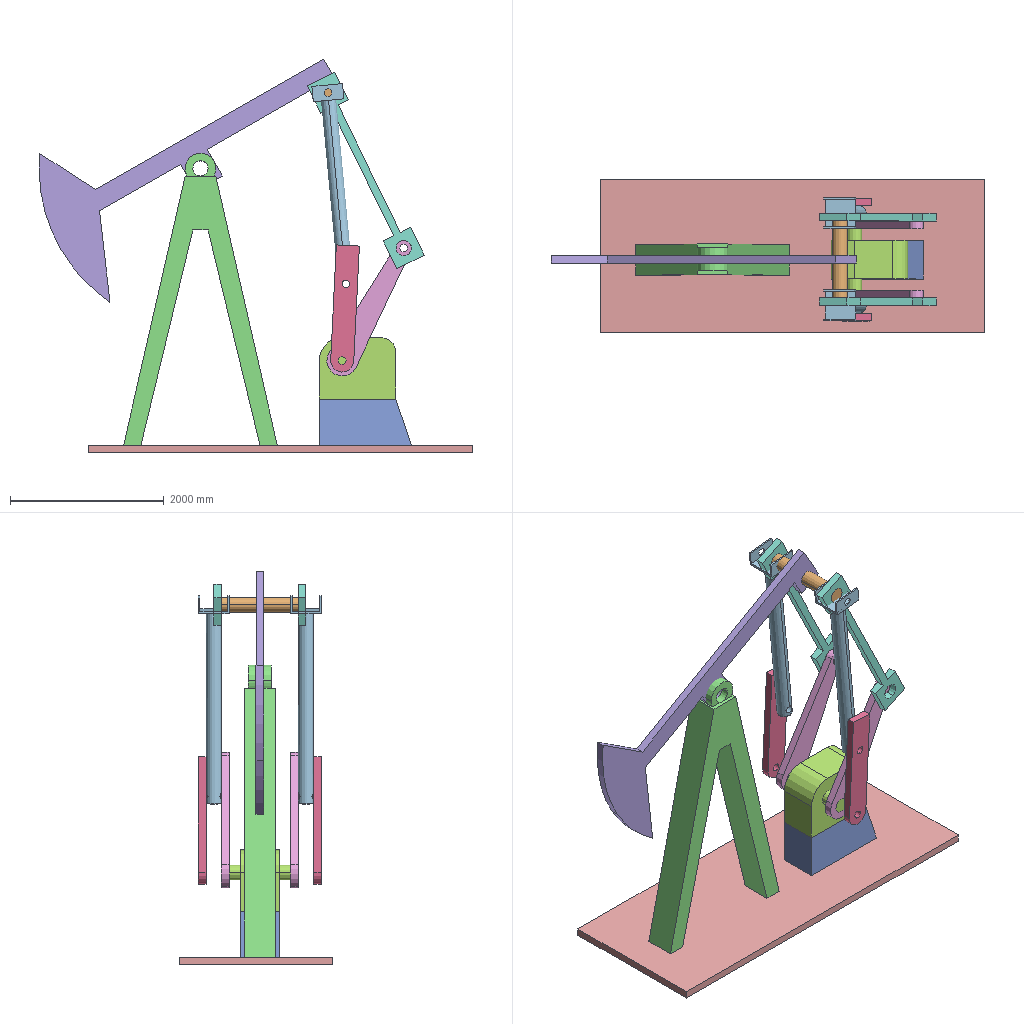Assembly | SolidWorks | 10 different items | 14 placed | box 5644 x 2000 x 5123 mm
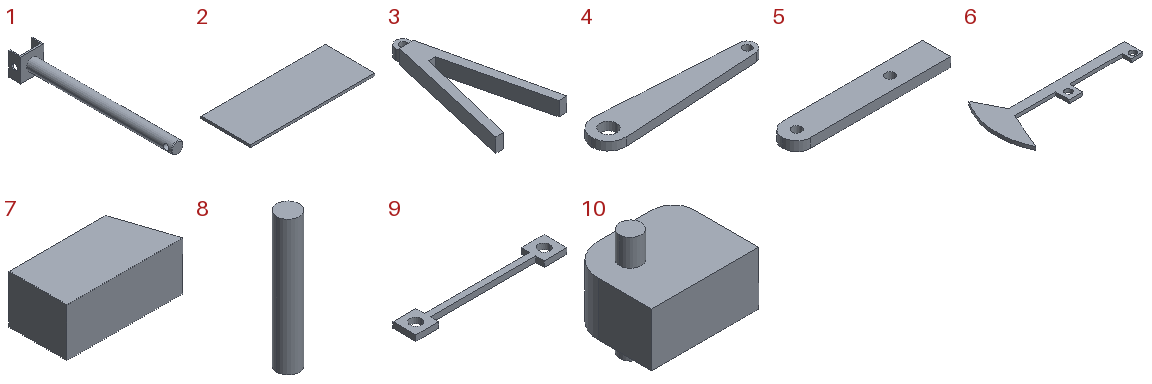Parts list (item | quantity | size | volume | features):
1 | x2 | 400 x 2700 x 400 mm | 84212442 mm3 | features ICE 3, Extrusion 1, Fillet 1
2 | x1 | 5000 x 2000 x 100 mm | 1000000000 mm3 | features Extrusion 1
3 | x1 | 2000 x 3800 x 400 mm | 719938598 mm3 | features ICE 2, Extrusion 1
4 | x2 | 1970 x 400 x 100 mm | 54116838 mm3 | features Extrusion 1
5 | x2 | 1650 x 300 x 100 mm | 46963495 mm3 | features Extrusion 1
6 | x1 | 4200 x 2133 x 100 mm | 203520372 mm3 | features Extrusion 1, ICE 1
7 | x1 | 1200 x 600 x 500 mm | 330000000 mm3 | features Extrusion 1
8 | x1 | 200 x 200 x 1200 mm | 37699112 mm3 | features Extrusion 1
9 | x2 | 2650 x 400 x 100 mm | 44216815 mm3 | features Extrusion 1
10 | x1 | 1000 x 800 x 1000 mm | 401758844 mm3 | features Fillet 2, Extrusion 1, ICE 1
Mates (type | each side: item.copy, entity, surface, feature):
Coincident | 2.1 face plane Boss-Extrude1 | 7.1 face plane Boss-Extrude1
DistanceDim | 7.1 face plane Boss-Extrude1 | 2.1 face plane Boss-Extrude1 | 2 times
Coincident | 7.1 face plane Boss-Extrude1 | 10.1 face plane Boss-Extrude1 | 3 times
Concentric | 10.1 face cylinder Boss-Extrude2 | 4.1 face cylinder Boss-Extrude1
Coincident | 10.1 face plane Boss-Extrude2 | 4.1 face plane Boss-Extrude1
Concentric | 10.1 face cylinder Boss-Extrude2 | 4.2 face cylinder Boss-Extrude1
Coincident | 10.1 face plane Boss-Extrude2 | 4.2 face plane Boss-Extrude1
Coincident | 4.1 face plane Boss-Extrude1 | 4.2 face plane Boss-Extrude1
Concentric | 4.1 face cylinder Boss-Extrude1 | 9.1 face cylinder Boss-Extrude1
Coincident | 4.1 face plane Boss-Extrude1 | 9.1 face plane Boss-Extrude1
Concentric | 4.2 face cylinder Boss-Extrude1 | 9.2 face cylinder Boss-Extrude1
Coincident | 4.2 face plane Boss-Extrude1 | 9.2 face plane Boss-Extrude1
Concentric | 9.1 face cylinder Boss-Extrude1 | 8.1 face cylinder Boss-Extrude1
Concentric | 9.2 face cylinder Boss-Extrude1 | 8.1 face cylinder Boss-Extrude1
Coincident | 9.2 face plane Boss-Extrude1 | 8.1 face plane Boss-Extrude1
Concentric | 8.1 face cylinder Boss-Extrude1 | 6.1 face cylinder Cut-Extrude1
DistanceDim | 6.1 face plane Boss-Extrude1 | 9.2 face plane Boss-Extrude1
Coincident | 2.1 face plane Boss-Extrude1 | 3.1 face plane Boss-Extrude2
Coincident | 10.1 plane | 3.1 plane
Concentric | 6.1 face cylinder Cut-Extrude1 | 3.1 face cylinder Boss-Extrude1
DistanceDim | 3.1 plane | 10.1 plane
Concentric | 10.1 face cylinder Boss-Extrude2 | 5.1 face cylinder Boss-Extrude1
DistanceDim | 5.1 face plane Boss-Extrude1 | 4.1 face plane Boss-Extrude1
Concentric | 10.1 face cylinder Boss-Extrude2 | 5.2 face cylinder Boss-Extrude1
DistanceDim | 5.2 face plane Boss-Extrude1 | 10.1 face plane Boss-Extrude2
Coincident | 5.1 face plane Boss-Extrude1 | 5.2 face plane Boss-Extrude1
Concentric | 8.1 face cylinder Boss-Extrude1 | 1.1 face cylinder Cut-Extrude1
DistanceDim | 1.1 face plane Boss-Extrude1 | 9.2 face plane Boss-Extrude1
Concentric | 5.2 face cylinder Boss-Extrude1 | 1.1 face cylinder Cut-Extrude2
Concentric | 8.1 face cylinder Boss-Extrude1 | 1.2 face cylinder Cut-Extrude1
DistanceDim | 1.2 face plane Boss-Extrude1 | 9.1 face plane Boss-Extrude1
Concentric | 5.1 face cylinder Boss-Extrude1 | 1.2 face cylinder Cut-Extrude2